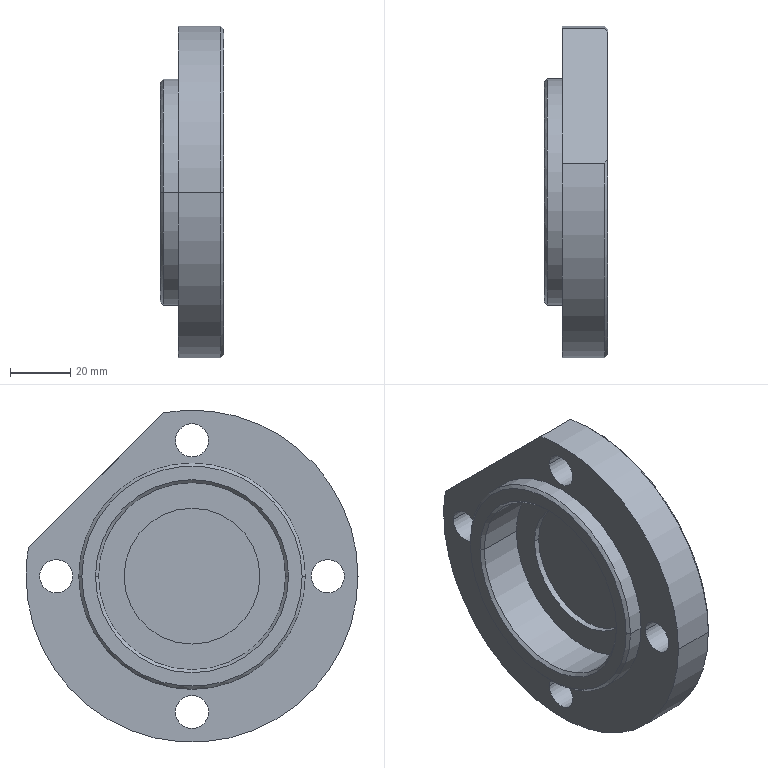Part | SolidWorks | features BaseBody 1 | 1 solid | 30 faces | box 21 x 110 x 110 mm | volume 105066 mm3 | cylinder 17 | cone 7 | plane 6 | commonest cylinder face diameters 11 x8 110 x3 45 x2 62 x2 75 x2
STEP:
#1=CARTESIAN_POINT('',(0.,-5.5,-45.));
#2=VERTEX_POINT('',#1);
#3=CARTESIAN_POINT('',(0.,5.5,-45.));
#4=VERTEX_POINT('',#3);
#5=CARTESIAN_POINT('',(0.,0.,-45.));
#6=DIRECTION('',(1.,0.,0.));
#7=DIRECTION('',(0.,1.,0.));
#8=AXIS2_PLACEMENT_3D('',#5,#6,#7);
#9=CIRCLE('',#8,5.5);
#10=EDGE_CURVE('',#2,#4,#9,.T.);
#11=ORIENTED_EDGE('',*,*,#10,.F.);
#12=CARTESIAN_POINT('',(15.,-5.5,-45.));
#13=VERTEX_POINT('',#12);
#14=CARTESIAN_POINT('',(-141.975,-5.5,-45.));
#15=DIRECTION('',(1.,0.,0.));
#16=VECTOR('',#15,1000.);
#17=LINE('',#14,#16);
#18=EDGE_CURVE('',#2,#13,#17,.T.);
#19=ORIENTED_EDGE('',*,*,#18,.T.);
#20=CARTESIAN_POINT('',(15.,5.5,-45.));
#21=VERTEX_POINT('',#20);
#22=CARTESIAN_POINT('',(15.,0.,-45.));
#23=DIRECTION('',(-1.,0.,0.));
#24=DIRECTION('',(0.,1.,0.));
#25=AXIS2_PLACEMENT_3D('',#22,#23,#24);
#26=CIRCLE('',#25,5.5);
#27=EDGE_CURVE('',#21,#13,#26,.T.);
#28=ORIENTED_EDGE('',*,*,#27,.F.);
#29=CARTESIAN_POINT('',(-141.975,5.5,-45.));
#30=DIRECTION('',(1.,0.,0.));
#31=VECTOR('',#30,1000.);
#32=LINE('',#29,#31);
#33=EDGE_CURVE('',#4,#21,#32,.T.);
#34=ORIENTED_EDGE('',*,*,#33,.F.);
#35=EDGE_LOOP('',(#11,#19,#28,#34));
#36=FACE_OUTER_BOUND('',#35,.T.);
#37=CARTESIAN_POINT('',(-141.975,0.,-45.));
#38=DIRECTION('',(1.,0.,0.));
#39=DIRECTION('',(0.,1.,0.));
#40=AXIS2_PLACEMENT_3D('',#37,#38,#39);
#41=CYLINDRICAL_SURFACE('',#40,5.5);
#42=ADVANCED_FACE('',(#36),#41,.F.);
#43=CARTESIAN_POINT('',(0.,-50.5,0.));
#44=VERTEX_POINT('',#43);
#45=CARTESIAN_POINT('',(0.,-39.5,0.));
#46=VERTEX_POINT('',#45);
#47=CARTESIAN_POINT('',(0.,-45.,0.));
#48=DIRECTION('',(1.,0.,0.));
#49=DIRECTION('',(0.,1.,0.));
#50=AXIS2_PLACEMENT_3D('',#47,#48,#49);
#51=CIRCLE('',#50,5.5);
#52=EDGE_CURVE('',#44,#46,#51,.T.);
#53=ORIENTED_EDGE('',*,*,#52,.F.);
#54=CARTESIAN_POINT('',(15.,-50.5,0.));
#55=VERTEX_POINT('',#54);
#56=CARTESIAN_POINT('',(-141.975,-50.5,0.));
#57=DIRECTION('',(1.,0.,0.));
#58=VECTOR('',#57,1000.);
#59=LINE('',#56,#58);
#60=EDGE_CURVE('',#44,#55,#59,.T.);
#61=ORIENTED_EDGE('',*,*,#60,.T.);
#62=CARTESIAN_POINT('',(15.,-39.5,0.));
#63=VERTEX_POINT('',#62);
#64=CARTESIAN_POINT('',(15.,-45.,0.));
#65=DIRECTION('',(-1.,0.,0.));
#66=DIRECTION('',(0.,1.,0.));
#67=AXIS2_PLACEMENT_3D('',#64,#65,#66);
#68=CIRCLE('',#67,5.5);
#69=EDGE_CURVE('',#63,#55,#68,.T.);
#70=ORIENTED_EDGE('',*,*,#69,.F.);
#71=CARTESIAN_POINT('',(-141.975,-39.5,0.));
#72=DIRECTION('',(1.,0.,0.));
#73=VECTOR('',#72,1000.);
#74=LINE('',#71,#73);
#75=EDGE_CURVE('',#46,#63,#74,.T.);
#76=ORIENTED_EDGE('',*,*,#75,.F.);
#77=EDGE_LOOP('',(#53,#61,#70,#76));
#78=FACE_OUTER_BOUND('',#77,.T.);
#79=CARTESIAN_POINT('',(-141.975,-45.,0.));
#80=DIRECTION('',(1.,0.,0.));
#81=DIRECTION('',(0.,1.,0.));
#82=AXIS2_PLACEMENT_3D('',#79,#80,#81);
#83=CYLINDRICAL_SURFACE('',#82,5.5);
#84=ADVANCED_FACE('',(#78),#83,.F.);
#85=CARTESIAN_POINT('',(0.,-5.5,45.));
#86=VERTEX_POINT('',#85);
#87=CARTESIAN_POINT('',(0.,5.5,45.));
#88=VERTEX_POINT('',#87);
#89=CARTESIAN_POINT('',(0.,0.,45.));
#90=DIRECTION('',(1.,0.,0.));
#91=DIRECTION('',(0.,1.,0.));
#92=AXIS2_PLACEMENT_3D('',#89,#90,#91);
#93=CIRCLE('',#92,5.5);
#94=EDGE_CURVE('',#86,#88,#93,.T.);
#95=ORIENTED_EDGE('',*,*,#94,.F.);
#96=CARTESIAN_POINT('',(15.,-5.5,45.));
#97=VERTEX_POINT('',#96);
#98=CARTESIAN_POINT('',(-141.975,-5.5,45.));
#99=DIRECTION('',(1.,0.,0.));
#100=VECTOR('',#99,1000.);
#101=LINE('',#98,#100);
#102=EDGE_CURVE('',#86,#97,#101,.T.);
#103=ORIENTED_EDGE('',*,*,#102,.T.);
#104=CARTESIAN_POINT('',(15.,5.5,45.));
#105=VERTEX_POINT('',#104);
#106=CARTESIAN_POINT('',(15.,0.,45.));
#107=DIRECTION('',(-1.,0.,0.));
#108=DIRECTION('',(0.,1.,0.));
#109=AXIS2_PLACEMENT_3D('',#106,#107,#108);
#110=CIRCLE('',#109,5.5);
#111=EDGE_CURVE('',#105,#97,#110,.T.);
#112=ORIENTED_EDGE('',*,*,#111,.F.);
#113=CARTESIAN_POINT('',(-141.975,5.5,45.));
#114=DIRECTION('',(1.,0.,0.));
#115=VECTOR('',#114,1000.);
#116=LINE('',#113,#115);
#117=EDGE_CURVE('',#88,#105,#116,.T.);
#118=ORIENTED_EDGE('',*,*,#117,.F.);
#119=EDGE_LOOP('',(#95,#103,#112,#118));
#120=FACE_OUTER_BOUND('',#119,.T.);
#121=CARTESIAN_POINT('',(-141.975,0.,45.));
#122=DIRECTION('',(1.,0.,0.));
#123=DIRECTION('',(0.,1.,0.));
#124=AXIS2_PLACEMENT_3D('',#121,#122,#123);
#125=CYLINDRICAL_SURFACE('',#124,5.5);
#126=ADVANCED_FACE('',(#120),#125,.F.);
#127=CARTESIAN_POINT('',(0.,39.5,0.));
#128=VERTEX_POINT('',#127);
#129=CARTESIAN_POINT('',(0.,50.5,0.));
#130=VERTEX_POINT('',#129);
#131=CARTESIAN_POINT('',(0.,45.,0.));
#132=DIRECTION('',(1.,0.,0.));
#133=DIRECTION('',(0.,1.,0.));
#134=AXIS2_PLACEMENT_3D('',#131,#132,#133);
#135=CIRCLE('',#134,5.5);
#136=EDGE_CURVE('',#128,#130,#135,.T.);
#137=ORIENTED_EDGE('',*,*,#136,.F.);
#138=CARTESIAN_POINT('',(15.,39.5,0.));
#139=VERTEX_POINT('',#138);
#140=CARTESIAN_POINT('',(-141.975,39.5,0.));
#141=DIRECTION('',(1.,0.,0.));
#142=VECTOR('',#141,1000.);
#143=LINE('',#140,#142);
#144=EDGE_CURVE('',#128,#139,#143,.T.);
#145=ORIENTED_EDGE('',*,*,#144,.T.);
#146=CARTESIAN_POINT('',(15.,50.5,0.));
#147=VERTEX_POINT('',#146);
#148=CARTESIAN_POINT('',(15.,45.,0.));
#149=DIRECTION('',(-1.,0.,0.));
#150=DIRECTION('',(0.,1.,0.));
#151=AXIS2_PLACEMENT_3D('',#148,#149,#150);
#152=CIRCLE('',#151,5.5);
#153=EDGE_CURVE('',#147,#139,#152,.T.);
#154=ORIENTED_EDGE('',*,*,#153,.F.);
#155=CARTESIAN_POINT('',(-141.975,50.5,0.));
#156=DIRECTION('',(1.,0.,0.));
#157=VECTOR('',#156,1000.);
#158=LINE('',#155,#157);
#159=EDGE_CURVE('',#130,#147,#158,.T.);
#160=ORIENTED_EDGE('',*,*,#159,.F.);
#161=EDGE_LOOP('',(#137,#145,#154,#160));
#162=FACE_OUTER_BOUND('',#161,.T.);
#163=CARTESIAN_POINT('',(-141.975,45.,0.));
#164=DIRECTION('',(1.,0.,0.));
#165=DIRECTION('',(0.,1.,0.));
#166=AXIS2_PLACEMENT_3D('',#163,#164,#165);
#167=CYLINDRICAL_SURFACE('',#166,5.5);
#168=ADVANCED_FACE('',(#162),#167,.F.);
#169=CARTESIAN_POINT('',(15.,54.,0.));
#170=VERTEX_POINT('',#169);
#171=CARTESIAN_POINT('',(15.,52.927,10.713));
#172=VERTEX_POINT('',#171);
#173=CARTESIAN_POINT('',(15.,0.,0.));
#174=DIRECTION('',(1.,0.,0.));
#175=DIRECTION('',(0.,-1.,0.));
#176=AXIS2_PLACEMENT_3D('',#173,#174,#175);
#177=CIRCLE('',#176,54.);
#178=EDGE_CURVE('',#170,#172,#177,.T.);
#179=ORIENTED_EDGE('',*,*,#178,.F.);
#180=CARTESIAN_POINT('',(14.,55.,0.));
#181=VERTEX_POINT('',#180);
#182=CARTESIAN_POINT('',(14.,55.,0.));
#183=DIRECTION('',(-0.7071,0.7071,0.));
#184=VECTOR('',#183,1000.);
#185=LINE('',#182,#184);
#186=EDGE_CURVE('',#170,#181,#185,.T.);
#187=ORIENTED_EDGE('',*,*,#186,.T.);
#188=CARTESIAN_POINT('',(14.,54.18,9.459));
#189=VERTEX_POINT('',#188);
#190=CARTESIAN_POINT('',(14.,0.,0.));
#191=DIRECTION('',(1.,0.,0.));
#192=DIRECTION('',(0.,-1.,0.));
#193=AXIS2_PLACEMENT_3D('',#190,#191,#192);
#194=CIRCLE('',#193,55.);
#195=EDGE_CURVE('',#181,#189,#194,.T.);
#196=ORIENTED_EDGE('',*,*,#195,.T.);
#197=CARTESIAN_POINT('',(14.,54.18,9.459));
#198=CARTESIAN_POINT('',(14.338,53.765,9.875));
#199=CARTESIAN_POINT('',(14.672,53.347,10.293));
#200=CARTESIAN_POINT('',(15.,52.927,10.713));
#201=B_SPLINE_CURVE_WITH_KNOTS('',3,(#197,#198,#199,#200),.UNSPECIFIED.,.F.,.F.,(4,4),(0.,0.002036),.UNSPECIFIED.);
#202=EDGE_CURVE('',#189,#172,#201,.T.);
#203=ORIENTED_EDGE('',*,*,#202,.T.);
#204=EDGE_LOOP('',(#179,#187,#196,#203));
#205=FACE_OUTER_BOUND('',#204,.T.);
#206=CARTESIAN_POINT('',(14.,0.,0.));
#207=DIRECTION('',(-1.,0.,0.));
#208=DIRECTION('',(0.,-1.,0.));
#209=AXIS2_PLACEMENT_3D('',#206,#207,#208);
#210=CONICAL_SURFACE('',#209,55.,0.7854);
#211=ADVANCED_FACE('',(#205),#210,.T.);
#212=ORIENTED_EDGE('',*,*,#186,.F.);
#213=CARTESIAN_POINT('',(15.,-54.,0.));
#214=VERTEX_POINT('',#213);
#215=CARTESIAN_POINT('',(15.,0.,0.));
#216=DIRECTION('',(1.,0.,0.));
#217=DIRECTION('',(0.,-1.,0.));
#218=AXIS2_PLACEMENT_3D('',#215,#216,#217);
#219=CIRCLE('',#218,54.);
#220=EDGE_CURVE('',#214,#170,#219,.T.);
#221=ORIENTED_EDGE('',*,*,#220,.F.);
#222=CARTESIAN_POINT('',(14.,-55.,0.));
#223=VERTEX_POINT('',#222);
#224=CARTESIAN_POINT('',(14.,-55.,0.));
#225=DIRECTION('',(-0.7071,-0.7071,0.));
#226=VECTOR('',#225,1000.);
#227=LINE('',#224,#226);
#228=EDGE_CURVE('',#214,#223,#227,.T.);
#229=ORIENTED_EDGE('',*,*,#228,.T.);
#230=CARTESIAN_POINT('',(14.,0.,0.));
#231=DIRECTION('',(1.,0.,0.));
#232=DIRECTION('',(0.,-1.,0.));
#233=AXIS2_PLACEMENT_3D('',#230,#231,#232);
#234=CIRCLE('',#233,55.);
#235=EDGE_CURVE('',#223,#181,#234,.T.);
#236=ORIENTED_EDGE('',*,*,#235,.T.);
#237=EDGE_LOOP('',(#212,#221,#229,#236));
#238=FACE_OUTER_BOUND('',#237,.T.);
#239=CARTESIAN_POINT('',(14.,0.,0.));
#240=DIRECTION('',(-1.,0.,0.));
#241=DIRECTION('',(0.,-1.,0.));
#242=AXIS2_PLACEMENT_3D('',#239,#240,#241);
#243=CONICAL_SURFACE('',#242,55.,0.7854);
#244=ADVANCED_FACE('',(#238),#243,.T.);
#245=CARTESIAN_POINT('',(0.,-55.,0.));
#246=VERTEX_POINT('',#245);
#247=CARTESIAN_POINT('',(0.,9.459,54.18));
#248=VERTEX_POINT('',#247);
#249=CARTESIAN_POINT('',(0.,0.,0.));
#250=DIRECTION('',(-1.,0.,0.));
#251=DIRECTION('',(0.,1.,0.));
#252=AXIS2_PLACEMENT_3D('',#249,#250,#251);
#253=CIRCLE('',#252,55.);
#254=EDGE_CURVE('',#246,#248,#253,.T.);
#255=ORIENTED_EDGE('',*,*,#254,.F.);
#256=CARTESIAN_POINT('',(7.5,-55.,0.));
#257=DIRECTION('',(1.,0.,0.));
#258=VECTOR('',#257,1000.);
#259=LINE('',#256,#258);
#260=EDGE_CURVE('',#246,#223,#259,.T.);
#261=ORIENTED_EDGE('',*,*,#260,.T.);
#262=CARTESIAN_POINT('',(14.,9.459,54.18));
#263=VERTEX_POINT('',#262);
#264=CARTESIAN_POINT('',(14.,0.,0.));
#265=DIRECTION('',(1.,0.,0.));
#266=DIRECTION('',(0.,-1.,0.));
#267=AXIS2_PLACEMENT_3D('',#264,#265,#266);
#268=CIRCLE('',#267,55.);
#269=EDGE_CURVE('',#263,#223,#268,.T.);
#270=ORIENTED_EDGE('',*,*,#269,.F.);
#271=CARTESIAN_POINT('',(15.,9.459,54.18));
#272=DIRECTION('',(-1.,0.,0.));
#273=VECTOR('',#272,1000.);
#274=LINE('',#271,#273);
#275=EDGE_CURVE('',#263,#248,#274,.T.);
#276=ORIENTED_EDGE('',*,*,#275,.T.);
#277=EDGE_LOOP('',(#255,#261,#270,#276));
#278=FACE_OUTER_BOUND('',#277,.T.);
#279=CARTESIAN_POINT('',(7.5,0.,0.));
#280=DIRECTION('',(1.,0.,0.));
#281=DIRECTION('',(0.,1.,0.));
#282=AXIS2_PLACEMENT_3D('',#279,#280,#281);
#283=CYLINDRICAL_SURFACE('',#282,55.);
#284=ADVANCED_FACE('',(#278),#283,.T.);
#285=ORIENTED_EDGE('',*,*,#260,.F.);
#286=CARTESIAN_POINT('',(0.,55.,0.));
#287=VERTEX_POINT('',#286);
#288=CARTESIAN_POINT('',(0.,0.,0.));
#289=DIRECTION('',(-1.,0.,0.));
#290=DIRECTION('',(0.,1.,0.));
#291=AXIS2_PLACEMENT_3D('',#288,#289,#290);
#292=CIRCLE('',#291,55.);
#293=EDGE_CURVE('',#287,#246,#292,.T.);
#294=ORIENTED_EDGE('',*,*,#293,.F.);
#295=CARTESIAN_POINT('',(7.5,55.,0.));
#296=DIRECTION('',(1.,0.,0.));
#297=VECTOR('',#296,1000.);
#298=LINE('',#295,#297);
#299=EDGE_CURVE('',#287,#181,#298,.T.);
#300=ORIENTED_EDGE('',*,*,#299,.T.);
#301=ORIENTED_EDGE('',*,*,#235,.F.);
#302=EDGE_LOOP('',(#285,#294,#300,#301));
#303=FACE_OUTER_BOUND('',#302,.T.);
#304=CARTESIAN_POINT('',(7.5,0.,0.));
#305=DIRECTION('',(1.,0.,0.));
#306=DIRECTION('',(0.,1.,0.));
#307=AXIS2_PLACEMENT_3D('',#304,#305,#306);
#308=CYLINDRICAL_SURFACE('',#307,55.);
#309=ADVANCED_FACE('',(#303),#308,.T.);
#310=CARTESIAN_POINT('',(-5.,37.5,0.));
#311=VERTEX_POINT('',#310);
#312=CARTESIAN_POINT('',(-5.,-37.5,0.));
#313=VERTEX_POINT('',#312);
#314=CARTESIAN_POINT('',(-5.,0.,0.));
#315=DIRECTION('',(1.,0.,0.));
#316=DIRECTION('',(0.,1.,0.));
#317=AXIS2_PLACEMENT_3D('',#314,#315,#316);
#318=CIRCLE('',#317,37.5);
#319=EDGE_CURVE('',#311,#313,#318,.T.);
#320=ORIENTED_EDGE('',*,*,#319,.T.);
#321=CARTESIAN_POINT('',(0.,-37.5,0.));
#322=VERTEX_POINT('',#321);
#323=CARTESIAN_POINT('',(-3.,-37.5,0.));
#324=DIRECTION('',(1.,0.,0.));
#325=VECTOR('',#324,1000.);
#326=LINE('',#323,#325);
#327=EDGE_CURVE('',#313,#322,#326,.T.);
#328=ORIENTED_EDGE('',*,*,#327,.T.);
#329=CARTESIAN_POINT('',(0.,37.5,0.));
#330=VERTEX_POINT('',#329);
#331=CARTESIAN_POINT('',(0.,0.,0.));
#332=DIRECTION('',(1.,0.,0.));
#333=DIRECTION('',(0.,1.,0.));
#334=AXIS2_PLACEMENT_3D('',#331,#332,#333);
#335=CIRCLE('',#334,37.5);
#336=EDGE_CURVE('',#330,#322,#335,.T.);
#337=ORIENTED_EDGE('',*,*,#336,.F.);
#338=CARTESIAN_POINT('',(-3.,37.5,0.));
#339=DIRECTION('',(1.,0.,0.));
#340=VECTOR('',#339,1000.);
#341=LINE('',#338,#340);
#342=EDGE_CURVE('',#311,#330,#341,.T.);
#343=ORIENTED_EDGE('',*,*,#342,.F.);
#344=EDGE_LOOP('',(#320,#328,#337,#343));
#345=FACE_OUTER_BOUND('',#344,.T.);
#346=CARTESIAN_POINT('',(-3.,0.,0.));
#347=DIRECTION('',(1.,0.,0.));
#348=DIRECTION('',(0.,1.,0.));
#349=AXIS2_PLACEMENT_3D('',#346,#347,#348);
#350=CYLINDRICAL_SURFACE('',#349,37.5);
#351=ADVANCED_FACE('',(#345),#350,.T.);
#352=CARTESIAN_POINT('',(-6.,36.5,0.));
#353=VERTEX_POINT('',#352);
#354=CARTESIAN_POINT('',(-6.,-36.5,0.));
#355=VERTEX_POINT('',#354);
#356=CARTESIAN_POINT('',(-6.,0.,0.));
#357=DIRECTION('',(1.,0.,0.));
#358=DIRECTION('',(0.,1.,0.));
#359=AXIS2_PLACEMENT_3D('',#356,#357,#358);
#360=CIRCLE('',#359,36.5);
#361=EDGE_CURVE('',#353,#355,#360,.T.);
#362=ORIENTED_EDGE('',*,*,#361,.T.);
#363=CARTESIAN_POINT('',(-5.,-37.5,0.));
#364=DIRECTION('',(0.7071,-0.7071,0.));
#365=VECTOR('',#364,1000.);
#366=LINE('',#363,#365);
#367=EDGE_CURVE('',#355,#313,#366,.T.);
#368=ORIENTED_EDGE('',*,*,#367,.T.);
#369=ORIENTED_EDGE('',*,*,#319,.F.);
#370=CARTESIAN_POINT('',(-5.,37.5,0.));
#371=DIRECTION('',(0.7071,0.7071,0.));
#372=VECTOR('',#371,1000.);
#373=LINE('',#370,#372);
#374=EDGE_CURVE('',#353,#311,#373,.T.);
#375=ORIENTED_EDGE('',*,*,#374,.F.);
#376=EDGE_LOOP('',(#362,#368,#369,#375));
#377=FACE_OUTER_BOUND('',#376,.T.);
#378=CARTESIAN_POINT('',(-5.,0.,0.));
#379=DIRECTION('',(1.,0.,0.));
#380=DIRECTION('',(0.,1.,0.));
#381=AXIS2_PLACEMENT_3D('',#378,#379,#380);
#382=CONICAL_SURFACE('',#381,37.5,0.7854);
#383=ADVANCED_FACE('',(#377),#382,.T.);
#384=CARTESIAN_POINT('',(-5.,31.,0.));
#385=VERTEX_POINT('',#384);
#386=CARTESIAN_POINT('',(-5.,-31.,0.));
#387=VERTEX_POINT('',#386);
#388=CARTESIAN_POINT('',(-5.,0.,0.));
#389=DIRECTION('',(-1.,0.,0.));
#390=DIRECTION('',(0.,-1.,0.));
#391=AXIS2_PLACEMENT_3D('',#388,#389,#390);
#392=CIRCLE('',#391,31.);
#393=EDGE_CURVE('',#385,#387,#392,.T.);
#394=ORIENTED_EDGE('',*,*,#393,.F.);
#395=CARTESIAN_POINT('',(-6.,32.,0.));
#396=VERTEX_POINT('',#395);
#397=CARTESIAN_POINT('',(-6.,32.,0.));
#398=DIRECTION('',(-0.7071,0.7071,0.));
#399=VECTOR('',#398,1000.);
#400=LINE('',#397,#399);
#401=EDGE_CURVE('',#385,#396,#400,.T.);
#402=ORIENTED_EDGE('',*,*,#401,.T.);
#403=CARTESIAN_POINT('',(-6.,-32.,0.));
#404=VERTEX_POINT('',#403);
#405=CARTESIAN_POINT('',(-6.,0.,0.));
#406=DIRECTION('',(1.,0.,0.));
#407=DIRECTION('',(0.,-1.,0.));
#408=AXIS2_PLACEMENT_3D('',#405,#406,#407);
#409=CIRCLE('',#408,32.);
#410=EDGE_CURVE('',#404,#396,#409,.T.);
#411=ORIENTED_EDGE('',*,*,#410,.F.);
#412=CARTESIAN_POINT('',(-6.,-32.,0.));
#413=DIRECTION('',(-0.7071,-0.7071,0.));
#414=VECTOR('',#413,1000.);
#415=LINE('',#412,#414);
#416=EDGE_CURVE('',#387,#404,#415,.T.);
#417=ORIENTED_EDGE('',*,*,#416,.F.);
#418=EDGE_LOOP('',(#394,#402,#411,#417));
#419=FACE_OUTER_BOUND('',#418,.T.);
#420=CARTESIAN_POINT('',(-6.,0.,0.));
#421=DIRECTION('',(-1.,0.,0.));
#422=DIRECTION('',(0.,-1.,0.));
#423=AXIS2_PLACEMENT_3D('',#420,#421,#422);
#424=CONICAL_SURFACE('',#423,32.,0.7854);
#425=ADVANCED_FACE('',(#419),#424,.F.);
#426=ORIENTED_EDGE('',*,*,#393,.T.);
#427=CARTESIAN_POINT('',(10.,-31.,0.));
#428=VERTEX_POINT('',#427);
#429=CARTESIAN_POINT('',(2.,-31.,0.));
#430=DIRECTION('',(1.,0.,0.));
#431=VECTOR('',#430,1000.);
#432=LINE('',#429,#431);
#433=EDGE_CURVE('',#387,#428,#432,.T.);
#434=ORIENTED_EDGE('',*,*,#433,.T.);
#435=CARTESIAN_POINT('',(10.,31.,0.));
#436=VERTEX_POINT('',#435);
#437=CARTESIAN_POINT('',(10.,0.,0.));
#438=DIRECTION('',(-1.,0.,0.));
#439=DIRECTION('',(0.,1.,0.));
#440=AXIS2_PLACEMENT_3D('',#437,#438,#439);
#441=CIRCLE('',#440,31.);
#442=EDGE_CURVE('',#436,#428,#441,.T.);
#443=ORIENTED_EDGE('',*,*,#442,.F.);
#444=CARTESIAN_POINT('',(2.,31.,0.));
#445=DIRECTION('',(1.,0.,0.));
#446=VECTOR('',#445,1000.);
#447=LINE('',#444,#446);
#448=EDGE_CURVE('',#385,#436,#447,.T.);
#449=ORIENTED_EDGE('',*,*,#448,.F.);
#450=EDGE_LOOP('',(#426,#434,#443,#449));
#451=FACE_OUTER_BOUND('',#450,.T.);
#452=CARTESIAN_POINT('',(2.,0.,0.));
#453=DIRECTION('',(1.,0.,0.));
#454=DIRECTION('',(0.,1.,0.));
#455=AXIS2_PLACEMENT_3D('',#452,#453,#454);
#456=CYLINDRICAL_SURFACE('',#455,31.);
#457=ADVANCED_FACE('',(#451),#456,.F.);
#458=CARTESIAN_POINT('',(10.,-22.5,0.));
#459=VERTEX_POINT('',#458);
#460=CARTESIAN_POINT('',(10.,22.5,0.));
#461=VERTEX_POINT('',#460);
#462=CARTESIAN_POINT('',(10.,0.,0.));
#463=DIRECTION('',(1.,0.,0.));
#464=DIRECTION('',(0.,1.,0.));
#465=AXIS2_PLACEMENT_3D('',#462,#463,#464);
#466=CIRCLE('',#465,22.5);
#467=EDGE_CURVE('',#459,#461,#466,.T.);
#468=ORIENTED_EDGE('',*,*,#467,.F.);
#469=CARTESIAN_POINT('',(12.,-22.5,0.));
#470=VERTEX_POINT('',#469);
#471=CARTESIAN_POINT('',(11.,-22.5,0.));
#472=DIRECTION('',(1.,0.,0.));
#473=VECTOR('',#472,1000.);
#474=LINE('',#471,#473);
#475=EDGE_CURVE('',#459,#470,#474,.T.);
#476=ORIENTED_EDGE('',*,*,#475,.T.);
#477=CARTESIAN_POINT('',(12.,22.5,0.));
#478=VERTEX_POINT('',#477);
#479=CARTESIAN_POINT('',(12.,0.,0.));
#480=DIRECTION('',(-1.,0.,0.));
#481=DIRECTION('',(0.,1.,0.));
#482=AXIS2_PLACEMENT_3D('',#479,#480,#481);
#483=CIRCLE('',#482,22.5);
#484=EDGE_CURVE('',#478,#470,#483,.T.);
#485=ORIENTED_EDGE('',*,*,#484,.F.);
#486=CARTESIAN_POINT('',(11.,22.5,0.));
#487=DIRECTION('',(1.,0.,0.));
#488=VECTOR('',#487,1000.);
#489=LINE('',#486,#488);
#490=EDGE_CURVE('',#461,#478,#489,.T.);
#491=ORIENTED_EDGE('',*,*,#490,.F.);
#492=EDGE_LOOP('',(#468,#476,#485,#491));
#493=FACE_OUTER_BOUND('',#492,.T.);
#494=CARTESIAN_POINT('',(11.,0.,0.));
#495=DIRECTION('',(1.,0.,0.));
#496=DIRECTION('',(0.,1.,0.));
#497=AXIS2_PLACEMENT_3D('',#494,#495,#496);
#498=CYLINDRICAL_SURFACE('',#497,22.5);
#499=ADVANCED_FACE('',(#493),#498,.F.);
#500=ORIENTED_EDGE('',*,*,#27,.T.);
#501=CARTESIAN_POINT('',(15.,0.,-45.));
#502=DIRECTION('',(-1.,0.,0.));
#503=DIRECTION('',(0.,1.,0.));
#504=AXIS2_PLACEMENT_3D('',#501,#502,#503);
#505=CIRCLE('',#504,5.5);
#506=EDGE_CURVE('',#13,#21,#505,.T.);
#507=ORIENTED_EDGE('',*,*,#506,.T.);
#508=EDGE_LOOP('',(#500,#507));
#509=FACE_BOUND('',#508,.T.);
#510=ORIENTED_EDGE('',*,*,#69,.T.);
#511=CARTESIAN_POINT('',(15.,-45.,0.));
#512=DIRECTION('',(-1.,0.,0.));
#513=DIRECTION('',(0.,1.,0.));
#514=AXIS2_PLACEMENT_3D('',#511,#512,#513);
#515=CIRCLE('',#514,5.5);
#516=EDGE_CURVE('',#55,#63,#515,.T.);
#517=ORIENTED_EDGE('',*,*,#516,.T.);
#518=EDGE_LOOP('',(#510,#517));
#519=FACE_BOUND('',#518,.T.);
#520=ORIENTED_EDGE('',*,*,#111,.T.);
#521=CARTESIAN_POINT('',(15.,0.,45.));
#522=DIRECTION('',(-1.,0.,0.));
#523=DIRECTION('',(0.,1.,0.));
#524=AXIS2_PLACEMENT_3D('',#521,#522,#523);
#525=CIRCLE('',#524,5.5);
#526=EDGE_CURVE('',#97,#105,#525,.T.);
#527=ORIENTED_EDGE('',*,*,#526,.T.);
#528=EDGE_LOOP('',(#520,#527));
#529=FACE_BOUND('',#528,.T.);
#530=ORIENTED_EDGE('',*,*,#153,.T.);
#531=CARTESIAN_POINT('',(15.,45.,0.));
#532=DIRECTION('',(-1.,0.,0.));
#533=DIRECTION('',(0.,1.,0.));
#534=AXIS2_PLACEMENT_3D('',#531,#532,#533);
#535=CIRCLE('',#534,5.5);
#536=EDGE_CURVE('',#139,#147,#535,.T.);
#537=ORIENTED_EDGE('',*,*,#536,.T.);
#538=EDGE_LOOP('',(#530,#537));
#539=FACE_BOUND('',#538,.T.);
#540=CARTESIAN_POINT('',(15.,10.713,52.927));
#541=VERTEX_POINT('',#540);
#542=CARTESIAN_POINT('',(15.,52.927,10.713));
#543=DIRECTION('',(0.,-0.7071,0.7071));
#544=VECTOR('',#543,1000.);
#545=LINE('',#542,#544);
#546=EDGE_CURVE('',#172,#541,#545,.T.);
#547=ORIENTED_EDGE('',*,*,#546,.T.);
#548=CARTESIAN_POINT('',(15.,0.,0.));
#549=DIRECTION('',(1.,0.,0.));
#550=DIRECTION('',(0.,-1.,0.));
#551=AXIS2_PLACEMENT_3D('',#548,#549,#550);
#552=CIRCLE('',#551,54.);
#553=EDGE_CURVE('',#541,#214,#552,.T.);
#554=ORIENTED_EDGE('',*,*,#553,.T.);
#555=ORIENTED_EDGE('',*,*,#220,.T.);
#556=ORIENTED_EDGE('',*,*,#178,.T.);
#557=EDGE_LOOP('',(#547,#554,#555,#556));
#558=FACE_OUTER_BOUND('',#557,.T.);
#559=CARTESIAN_POINT('',(15.,0.,0.));
#560=DIRECTION('',(1.,0.,0.));
#561=DIRECTION('',(0.,1.,0.));
#562=AXIS2_PLACEMENT_3D('',#559,#560,#561);
#563=PLANE('',#562);
#564=ADVANCED_FACE('',(#509,#519,#529,#539,#558),#563,.T.);
#565=ORIENTED_EDGE('',*,*,#18,.F.);
#566=CARTESIAN_POINT('',(0.,0.,-45.));
#567=DIRECTION('',(1.,0.,0.));
#568=DIRECTION('',(0.,1.,0.));
#569=AXIS2_PLACEMENT_3D('',#566,#567,#568);
#570=CIRCLE('',#569,5.5);
#571=EDGE_CURVE('',#4,#2,#570,.T.);
#572=ORIENTED_EDGE('',*,*,#571,.F.);
#573=ORIENTED_EDGE('',*,*,#33,.T.);
#574=ORIENTED_EDGE('',*,*,#506,.F.);
#575=EDGE_LOOP('',(#565,#572,#573,#574));
#576=FACE_OUTER_BOUND('',#575,.T.);
#577=CARTESIAN_POINT('',(-141.975,0.,-45.));
#578=DIRECTION('',(1.,0.,0.));
#579=DIRECTION('',(0.,1.,0.));
#580=AXIS2_PLACEMENT_3D('',#577,#578,#579);
#581=CYLINDRICAL_SURFACE('',#580,5.5);
#582=ADVANCED_FACE('',(#576),#581,.F.);
#583=ORIENTED_EDGE('',*,*,#60,.F.);
#584=CARTESIAN_POINT('',(0.,-45.,0.));
#585=DIRECTION('',(1.,0.,0.));
#586=DIRECTION('',(0.,1.,0.));
#587=AXIS2_PLACEMENT_3D('',#584,#585,#586);
#588=CIRCLE('',#587,5.5);
#589=EDGE_CURVE('',#46,#44,#588,.T.);
#590=ORIENTED_EDGE('',*,*,#589,.F.);
#591=ORIENTED_EDGE('',*,*,#75,.T.);
#592=ORIENTED_EDGE('',*,*,#516,.F.);
#593=EDGE_LOOP('',(#583,#590,#591,#592));
#594=FACE_OUTER_BOUND('',#593,.T.);
#595=CARTESIAN_POINT('',(-141.975,-45.,0.));
#596=DIRECTION('',(1.,0.,0.));
#597=DIRECTION('',(0.,1.,0.));
#598=AXIS2_PLACEMENT_3D('',#595,#596,#597);
#599=CYLINDRICAL_SURFACE('',#598,5.5);
#600=ADVANCED_FACE('',(#594),#599,.F.);
#601=ORIENTED_EDGE('',*,*,#102,.F.);
#602=CARTESIAN_POINT('',(0.,0.,45.));
#603=DIRECTION('',(1.,0.,0.));
#604=DIRECTION('',(0.,1.,0.));
#605=AXIS2_PLACEMENT_3D('',#602,#603,#604);
#606=CIRCLE('',#605,5.5);
#607=EDGE_CURVE('',#88,#86,#606,.T.);
#608=ORIENTED_EDGE('',*,*,#607,.F.);
#609=ORIENTED_EDGE('',*,*,#117,.T.);
#610=ORIENTED_EDGE('',*,*,#526,.F.);
#611=EDGE_LOOP('',(#601,#608,#609,#610));
#612=FACE_OUTER_BOUND('',#611,.T.);
#613=CARTESIAN_POINT('',(-141.975,0.,45.));
#614=DIRECTION('',(1.,0.,0.));
#615=DIRECTION('',(0.,1.,0.));
#616=AXIS2_PLACEMENT_3D('',#613,#614,#615);
#617=CYLINDRICAL_SURFACE('',#616,5.5);
#618=ADVANCED_FACE('',(#612),#617,.F.);
#619=ORIENTED_EDGE('',*,*,#144,.F.);
#620=CARTESIAN_POINT('',(0.,45.,0.));
#621=DIRECTION('',(1.,0.,0.));
#622=DIRECTION('',(0.,1.,0.));
#623=AXIS2_PLACEMENT_3D('',#620,#621,#622);
#624=CIRCLE('',#623,5.5);
#625=EDGE_CURVE('',#130,#128,#624,.T.);
#626=ORIENTED_EDGE('',*,*,#625,.F.);
#627=ORIENTED_EDGE('',*,*,#159,.T.);
#628=ORIENTED_EDGE('',*,*,#536,.F.);
#629=EDGE_LOOP('',(#619,#626,#627,#628));
#630=FACE_OUTER_BOUND('',#629,.T.);
#631=CARTESIAN_POINT('',(-141.975,45.,0.));
#632=DIRECTION('',(1.,0.,0.));
#633=DIRECTION('',(0.,1.,0.));
#634=AXIS2_PLACEMENT_3D('',#631,#632,#633);
#635=CYLINDRICAL_SURFACE('',#634,5.5);
#636=ADVANCED_FACE('',(#630),#635,.F.);
#637=ORIENTED_EDGE('',*,*,#228,.F.);
#638=ORIENTED_EDGE('',*,*,#553,.F.);
#639=CARTESIAN_POINT('',(15.,10.713,52.927));
#640=CARTESIAN_POINT('',(14.672,10.293,53.347));
#641=CARTESIAN_POINT('',(14.338,9.875,53.765));
#642=CARTESIAN_POINT('',(14.,9.459,54.18));
#643=B_SPLINE_CURVE_WITH_KNOTS('',3,(#639,#640,#641,#642),.UNSPECIFIED.,.F.,.F.,(4,4),(0.,0.002036),.UNSPECIFIED.);
#644=EDGE_CURVE('',#541,#263,#643,.T.);
#645=ORIENTED_EDGE('',*,*,#644,.T.);
#646=ORIENTED_EDGE('',*,*,#269,.T.);
#647=EDGE_LOOP('',(#637,#638,#645,#646));
#648=FACE_OUTER_BOUND('',#647,.T.);
#649=CARTESIAN_POINT('',(14.,0.,0.));
#650=DIRECTION('',(-1.,0.,0.));
#651=DIRECTION('',(0.,-1.,0.));
#652=AXIS2_PLACEMENT_3D('',#649,#650,#651);
#653=CONICAL_SURFACE('',#652,55.,0.7854);
#654=ADVANCED_FACE('',(#648),#653,.T.);
#655=CARTESIAN_POINT('',(0.,54.18,9.459));
#656=VERTEX_POINT('',#655);
#657=CARTESIAN_POINT('',(15.,54.18,9.459));
#658=DIRECTION('',(1.,0.,0.));
#659=VECTOR('',#658,1000.);
#660=LINE('',#657,#659);
#661=EDGE_CURVE('',#656,#189,#660,.T.);
#662=ORIENTED_EDGE('',*,*,#661,.F.);
#663=CARTESIAN_POINT('',(0.,69.918,-6.278));
#664=DIRECTION('',(0.,0.7071,-0.7071));
#665=VECTOR('',#664,1000.);
#666=LINE('',#663,#665);
#667=EDGE_CURVE('',#248,#656,#666,.T.);
#668=ORIENTED_EDGE('',*,*,#667,.F.);
#669=ORIENTED_EDGE('',*,*,#275,.F.);
#670=ORIENTED_EDGE('',*,*,#644,.F.);
#671=ORIENTED_EDGE('',*,*,#546,.F.);
#672=ORIENTED_EDGE('',*,*,#202,.F.);
#673=EDGE_LOOP('',(#662,#668,#669,#670,#671,#672));
#674=FACE_OUTER_BOUND('',#673,.T.);
#675=CARTESIAN_POINT('',(15.,69.918,-6.278));
#676=DIRECTION('',(0.,-0.7071,-0.7071));
#677=DIRECTION('',(0.,0.7071,-0.7071));
#678=AXIS2_PLACEMENT_3D('',#675,#676,#677);
#679=PLANE('',#678);
#680=ADVANCED_FACE('',(#674),#679,.F.);
#681=ORIENTED_EDGE('',*,*,#336,.T.);
#682=CARTESIAN_POINT('',(0.,0.,0.));
#683=DIRECTION('',(1.,0.,0.));
#684=DIRECTION('',(0.,1.,0.));
#685=AXIS2_PLACEMENT_3D('',#682,#683,#684);
#686=CIRCLE('',#685,37.5);
#687=EDGE_CURVE('',#322,#330,#686,.T.);
#688=ORIENTED_EDGE('',*,*,#687,.T.);
#689=EDGE_LOOP('',(#681,#688));
#690=FACE_BOUND('',#689,.T.);
#691=ORIENTED_EDGE('',*,*,#625,.T.);
#692=ORIENTED_EDGE('',*,*,#136,.T.);
#693=EDGE_LOOP('',(#691,#692));
#694=FACE_BOUND('',#693,.T.);
#695=ORIENTED_EDGE('',*,*,#607,.T.);
#696=ORIENTED_EDGE('',*,*,#94,.T.);
#697=EDGE_LOOP('',(#695,#696));
#698=FACE_BOUND('',#697,.T.);
#699=ORIENTED_EDGE('',*,*,#589,.T.);
#700=ORIENTED_EDGE('',*,*,#52,.T.);
#701=EDGE_LOOP('',(#699,#700));
#702=FACE_BOUND('',#701,.T.);
#703=ORIENTED_EDGE('',*,*,#571,.T.);
#704=ORIENTED_EDGE('',*,*,#10,.T.);
#705=EDGE_LOOP('',(#703,#704));
#706=FACE_BOUND('',#705,.T.);
#707=ORIENTED_EDGE('',*,*,#667,.T.);
#708=CARTESIAN_POINT('',(0.,0.,0.));
#709=DIRECTION('',(-1.,0.,0.));
#710=DIRECTION('',(0.,1.,0.));
#711=AXIS2_PLACEMENT_3D('',#708,#709,#710);
#712=CIRCLE('',#711,55.);
#713=EDGE_CURVE('',#656,#287,#712,.T.);
#714=ORIENTED_EDGE('',*,*,#713,.T.);
#715=ORIENTED_EDGE('',*,*,#293,.T.);
#716=ORIENTED_EDGE('',*,*,#254,.T.);
#717=EDGE_LOOP('',(#707,#714,#715,#716));
#718=FACE_OUTER_BOUND('',#717,.T.);
#719=CARTESIAN_POINT('',(0.,55.,0.));
#720=DIRECTION('',(-1.,0.,0.));
#721=DIRECTION('',(0.,-1.,0.));
#722=AXIS2_PLACEMENT_3D('',#719,#720,#721);
#723=PLANE('',#722);
#724=ADVANCED_FACE('',(#690,#694,#698,#702,#706,#718),#723,.T.);
#725=ORIENTED_EDGE('',*,*,#299,.F.);
#726=ORIENTED_EDGE('',*,*,#713,.F.);
#727=ORIENTED_EDGE('',*,*,#661,.T.);
#728=ORIENTED_EDGE('',*,*,#195,.F.);
#729=EDGE_LOOP('',(#725,#726,#727,#728));
#730=FACE_OUTER_BOUND('',#729,.T.);
#731=CARTESIAN_POINT('',(7.5,0.,0.));
#732=DIRECTION('',(1.,0.,0.));
#733=DIRECTION('',(0.,1.,0.));
#734=AXIS2_PLACEMENT_3D('',#731,#732,#733);
#735=CYLINDRICAL_SURFACE('',#734,55.);
#736=ADVANCED_FACE('',(#730),#735,.T.);
#737=ORIENTED_EDGE('',*,*,#327,.F.);
#738=CARTESIAN_POINT('',(-5.,0.,0.));
#739=DIRECTION('',(1.,0.,0.));
#740=DIRECTION('',(0.,1.,0.));
#741=AXIS2_PLACEMENT_3D('',#738,#739,#740);
#742=CIRCLE('',#741,37.5);
#743=EDGE_CURVE('',#313,#311,#742,.T.);
#744=ORIENTED_EDGE('',*,*,#743,.T.);
#745=ORIENTED_EDGE('',*,*,#342,.T.);
#746=ORIENTED_EDGE('',*,*,#687,.F.);
#747=EDGE_LOOP('',(#737,#744,#745,#746));
#748=FACE_OUTER_BOUND('',#747,.T.);
#749=CARTESIAN_POINT('',(-3.,0.,0.));
#750=DIRECTION('',(1.,0.,0.));
#751=DIRECTION('',(0.,1.,0.));
#752=AXIS2_PLACEMENT_3D('',#749,#750,#751);
#753=CYLINDRICAL_SURFACE('',#752,37.5);
#754=ADVANCED_FACE('',(#748),#753,.T.);
#755=ORIENTED_EDGE('',*,*,#367,.F.);
#756=CARTESIAN_POINT('',(-6.,0.,0.));
#757=DIRECTION('',(1.,0.,0.));
#758=DIRECTION('',(0.,1.,0.));
#759=AXIS2_PLACEMENT_3D('',#756,#757,#758);
#760=CIRCLE('',#759,36.5);
#761=EDGE_CURVE('',#355,#353,#760,.T.);
#762=ORIENTED_EDGE('',*,*,#761,.T.);
#763=ORIENTED_EDGE('',*,*,#374,.T.);
#764=ORIENTED_EDGE('',*,*,#743,.F.);
#765=EDGE_LOOP('',(#755,#762,#763,#764));
#766=FACE_OUTER_BOUND('',#765,.T.);
#767=CARTESIAN_POINT('',(-5.,0.,0.));
#768=DIRECTION('',(1.,0.,0.));
#769=DIRECTION('',(0.,1.,0.));
#770=AXIS2_PLACEMENT_3D('',#767,#768,#769);
#771=CONICAL_SURFACE('',#770,37.5,0.7854);
#772=ADVANCED_FACE('',(#766),#771,.T.);
#773=ORIENTED_EDGE('',*,*,#410,.T.);
#774=CARTESIAN_POINT('',(-6.,0.,0.));
#775=DIRECTION('',(1.,0.,0.));
#776=DIRECTION('',(0.,-1.,0.));
#777=AXIS2_PLACEMENT_3D('',#774,#775,#776);
#778=CIRCLE('',#777,32.);
#779=EDGE_CURVE('',#396,#404,#778,.T.);
#780=ORIENTED_EDGE('',*,*,#779,.T.);
#781=EDGE_LOOP('',(#773,#780));
#782=FACE_BOUND('',#781,.T.);
#783=ORIENTED_EDGE('',*,*,#361,.F.);
#784=ORIENTED_EDGE('',*,*,#761,.F.);
#785=EDGE_LOOP('',(#783,#784));
#786=FACE_OUTER_BOUND('',#785,.T.);
#787=CARTESIAN_POINT('',(-6.,37.5,0.));
#788=DIRECTION('',(-1.,0.,0.));
#789=DIRECTION('',(0.,-1.,0.));
#790=AXIS2_PLACEMENT_3D('',#787,#788,#789);
#791=PLANE('',#790);
#792=ADVANCED_FACE('',(#782,#786),#791,.T.);
#793=ORIENTED_EDGE('',*,*,#401,.F.);
#794=CARTESIAN_POINT('',(-5.,0.,0.));
#795=DIRECTION('',(-1.,0.,0.));
#796=DIRECTION('',(0.,-1.,0.));
#797=AXIS2_PLACEMENT_3D('',#794,#795,#796);
#798=CIRCLE('',#797,31.);
#799=EDGE_CURVE('',#387,#385,#798,.T.);
#800=ORIENTED_EDGE('',*,*,#799,.F.);
#801=ORIENTED_EDGE('',*,*,#416,.T.);
#802=ORIENTED_EDGE('',*,*,#779,.F.);
#803=EDGE_LOOP('',(#793,#800,#801,#802));
#804=FACE_OUTER_BOUND('',#803,.T.);
#805=CARTESIAN_POINT('',(-6.,0.,0.));
#806=DIRECTION('',(-1.,0.,0.));
#807=DIRECTION('',(0.,-1.,0.));
#808=AXIS2_PLACEMENT_3D('',#805,#806,#807);
#809=CONICAL_SURFACE('',#808,32.,0.7854);
#810=ADVANCED_FACE('',(#804),#809,.F.);
#811=ORIENTED_EDGE('',*,*,#433,.F.);
#812=ORIENTED_EDGE('',*,*,#799,.T.);
#813=ORIENTED_EDGE('',*,*,#448,.T.);
#814=CARTESIAN_POINT('',(10.,0.,0.));
#815=DIRECTION('',(-1.,0.,0.));
#816=DIRECTION('',(0.,1.,0.));
#817=AXIS2_PLACEMENT_3D('',#814,#815,#816);
#818=CIRCLE('',#817,31.);
#819=EDGE_CURVE('',#428,#436,#818,.T.);
#820=ORIENTED_EDGE('',*,*,#819,.F.);
#821=EDGE_LOOP('',(#811,#812,#813,#820));
#822=FACE_OUTER_BOUND('',#821,.T.);
#823=CARTESIAN_POINT('',(2.,0.,0.));
#824=DIRECTION('',(1.,0.,0.));
#825=DIRECTION('',(0.,1.,0.));
#826=AXIS2_PLACEMENT_3D('',#823,#824,#825);
#827=CYLINDRICAL_SURFACE('',#826,31.);
#828=ADVANCED_FACE('',(#822),#827,.F.);
#829=CARTESIAN_POINT('',(10.,0.,0.));
#830=DIRECTION('',(1.,0.,0.));
#831=DIRECTION('',(0.,1.,0.));
#832=AXIS2_PLACEMENT_3D('',#829,#830,#831);
#833=CIRCLE('',#832,22.5);
#834=EDGE_CURVE('',#461,#459,#833,.T.);
#835=ORIENTED_EDGE('',*,*,#834,.T.);
#836=ORIENTED_EDGE('',*,*,#467,.T.);
#837=EDGE_LOOP('',(#835,#836));
#838=FACE_BOUND('',#837,.T.);
#839=ORIENTED_EDGE('',*,*,#442,.T.);
#840=ORIENTED_EDGE('',*,*,#819,.T.);
#841=EDGE_LOOP('',(#839,#840));
#842=FACE_OUTER_BOUND('',#841,.T.);
#843=CARTESIAN_POINT('',(10.,31.,0.));
#844=DIRECTION('',(-1.,0.,0.));
#845=DIRECTION('',(0.,-1.,0.));
#846=AXIS2_PLACEMENT_3D('',#843,#844,#845);
#847=PLANE('',#846);
#848=ADVANCED_FACE('',(#838,#842),#847,.T.);
#849=ORIENTED_EDGE('',*,*,#475,.F.);
#850=ORIENTED_EDGE('',*,*,#834,.F.);
#851=ORIENTED_EDGE('',*,*,#490,.T.);
#852=CARTESIAN_POINT('',(12.,0.,0.));
#853=DIRECTION('',(-1.,0.,0.));
#854=DIRECTION('',(0.,1.,0.));
#855=AXIS2_PLACEMENT_3D('',#852,#853,#854);
#856=CIRCLE('',#855,22.5);
#857=EDGE_CURVE('',#470,#478,#856,.T.);
#858=ORIENTED_EDGE('',*,*,#857,.F.);
#859=EDGE_LOOP('',(#849,#850,#851,#858));
#860=FACE_OUTER_BOUND('',#859,.T.);
#861=CARTESIAN_POINT('',(11.,0.,0.));
#862=DIRECTION('',(1.,0.,0.));
#863=DIRECTION('',(0.,1.,0.));
#864=AXIS2_PLACEMENT_3D('',#861,#862,#863);
#865=CYLINDRICAL_SURFACE('',#864,22.5);
#866=ADVANCED_FACE('',(#860),#865,.F.);
#867=ORIENTED_EDGE('',*,*,#484,.T.);
#868=ORIENTED_EDGE('',*,*,#857,.T.);
#869=EDGE_LOOP('',(#867,#868));
#870=FACE_OUTER_BOUND('',#869,.T.);
#871=CARTESIAN_POINT('',(12.,22.5,0.));
#872=DIRECTION('',(-1.,0.,0.));
#873=DIRECTION('',(0.,-1.,0.));
#874=AXIS2_PLACEMENT_3D('',#871,#872,#873);
#875=PLANE('',#874);
#876=ADVANCED_FACE('',(#870),#875,.T.);
#877=CLOSED_SHELL('',(#42,#84,#126,#168,#211,#244,#284,#309,#351,#383,#425,#457,#499,#564,#582,#600,#618,#636,#654,#680,#724,#736,#754,#772,#792,#810,#828,#848,#866,#876));
#878=MANIFOLD_SOLID_BREP('',#877);
#879=CARTESIAN_POINT('',(0.,0.,0.));
#880=DIRECTION('',(0.,0.,1.));
#881=DIRECTION('',(1.,0.,0.));
#882=AXIS2_PLACEMENT_3D('',#879,#880,#881);
#883=(LENGTH_UNIT()NAMED_UNIT(*)SI_UNIT(.MILLI.,.METRE.));
#884=UNCERTAINTY_MEASURE_WITH_UNIT(LENGTH_MEASURE(0.00001),#883,'','');
#885=(NAMED_UNIT(*)PLANE_ANGLE_UNIT()SI_UNIT($,.RADIAN.));
#886=(NAMED_UNIT(*)SI_UNIT($,.STERADIAN.)SOLID_ANGLE_UNIT());
#887=(GEOMETRIC_REPRESENTATION_CONTEXT(3)GLOBAL_UNCERTAINTY_ASSIGNED_CONTEXT((#884))GLOBAL_UNIT_ASSIGNED_CONTEXT((#883,#885,#886))REPRESENTATION_CONTEXT('',''));
#888=ADVANCED_BREP_SHAPE_REPRESENTATION('',(#878,#882),#887);